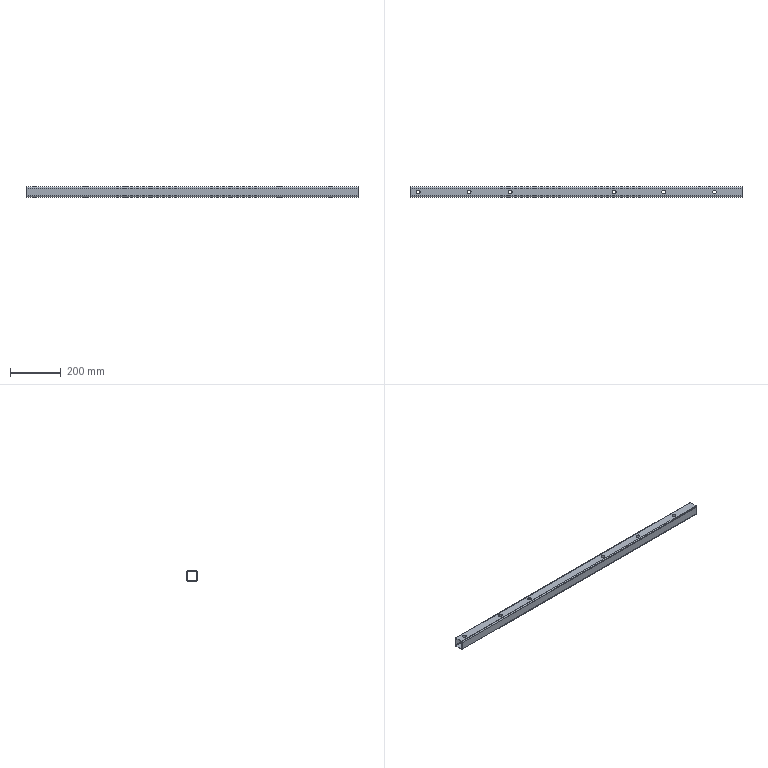Part | NX | features BREP 1 | 1 solid | 57 faces | box 1303 x 40 x 40 mm | volume 373746 mm3 | cylinder 40 | plane 17 | commonest cylinder face diameters 15 x24 6 x8 6.5 x4 10 x4